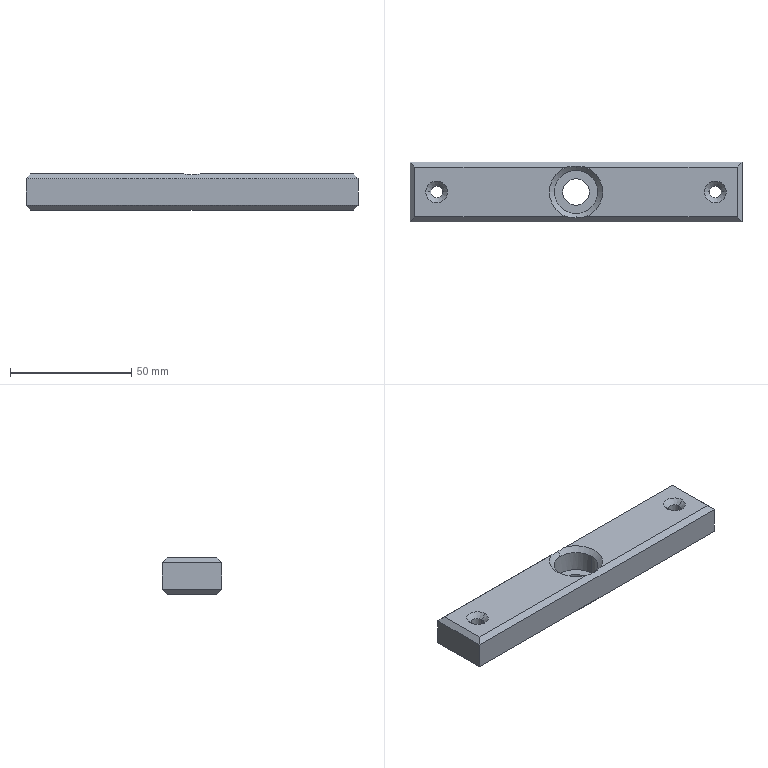Part | STEP file | Handle seat | 1 solid | 36 faces | box 137 x 24.5 x 15 mm | volume 45015 mm3 | plane 16 | cone 12 | cylinder 8 | commonest cylinder face diameters 5 x4 11 x2 18 x2